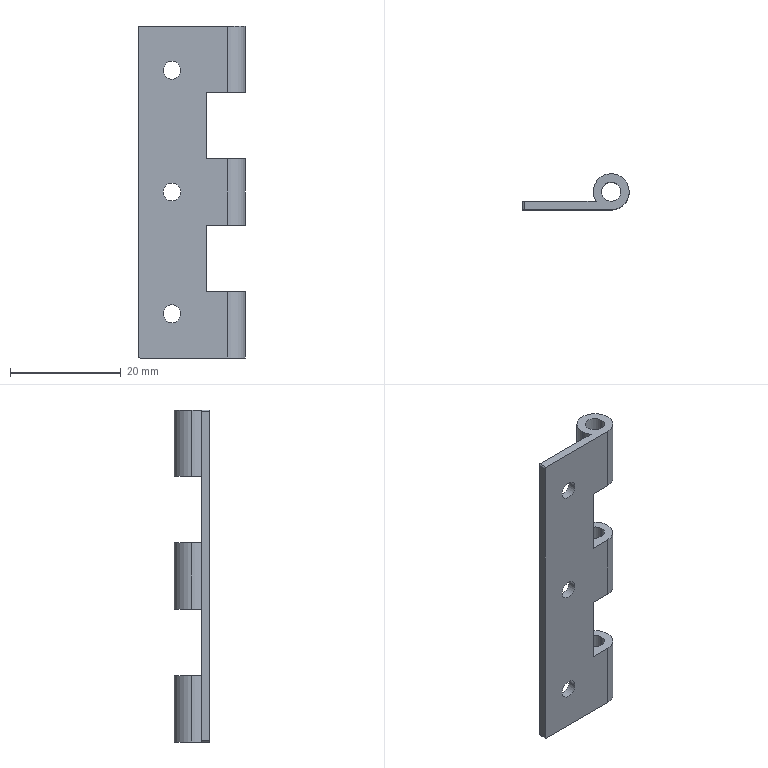Part | STEP file | Second B-1027-14 Pin A Part | 1 solid | 34 faces | box 19.25 x 6.5 x 60 mm | volume 2015 mm3 | cylinder 23 | plane 11 | commonest cylinder face diameters 6.5 x9 3.2 x6 3.5 x6 0.5 x2
STEP:
#1=CARTESIAN_POINT('',(-3.25,0.,-18.));
#2=VERTEX_POINT('',#1);
#3=CARTESIAN_POINT('',(3.25,0.,-18.));
#4=VERTEX_POINT('',#3);
#5=CARTESIAN_POINT('',(0.,0.,-18.));
#6=DIRECTION('',(0.,0.,-1.));
#7=DIRECTION('',(-1.,0.,0.));
#8=AXIS2_PLACEMENT_3D('',#5,#6,#7);
#9=CIRCLE('',#8,3.25);
#10=EDGE_CURVE('',#2,#4,#9,.T.);
#11=ORIENTED_EDGE('',*,*,#10,.T.);
#12=CARTESIAN_POINT('',(3.25,0.,-30.));
#13=VERTEX_POINT('',#12);
#14=CARTESIAN_POINT('',(3.25,0.,30.));
#15=DIRECTION('',(0.,0.,-1.));
#16=VECTOR('',#15,1000.);
#17=LINE('',#14,#16);
#18=EDGE_CURVE('',#4,#13,#17,.T.);
#19=ORIENTED_EDGE('',*,*,#18,.T.);
#20=CARTESIAN_POINT('',(-3.25,0.,-30.));
#21=VERTEX_POINT('',#20);
#22=CARTESIAN_POINT('',(0.,0.,-30.));
#23=DIRECTION('',(0.,0.,1.));
#24=DIRECTION('',(-1.,0.,0.));
#25=AXIS2_PLACEMENT_3D('',#22,#23,#24);
#26=CIRCLE('',#25,3.25);
#27=EDGE_CURVE('',#13,#21,#26,.T.);
#28=ORIENTED_EDGE('',*,*,#27,.T.);
#29=CARTESIAN_POINT('',(-3.25,0.,30.));
#30=DIRECTION('',(0.,0.,-1.));
#31=VECTOR('',#30,1000.);
#32=LINE('',#29,#31);
#33=EDGE_CURVE('',#2,#21,#32,.T.);
#34=ORIENTED_EDGE('',*,*,#33,.F.);
#35=EDGE_LOOP('',(#11,#19,#28,#34));
#36=FACE_OUTER_BOUND('',#35,.T.);
#37=CARTESIAN_POINT('',(0.,0.,30.));
#38=DIRECTION('',(0.,0.,-1.));
#39=DIRECTION('',(-1.,0.,0.));
#40=AXIS2_PLACEMENT_3D('',#37,#38,#39);
#41=CYLINDRICAL_SURFACE('',#40,3.25);
#42=ADVANCED_FACE('',(#36),#41,.T.);
#43=CARTESIAN_POINT('',(-2.739,-1.75,-18.));
#44=VERTEX_POINT('',#43);
#45=CARTESIAN_POINT('',(0.,0.,-18.));
#46=DIRECTION('',(0.,0.,-1.));
#47=DIRECTION('',(-1.,0.,0.));
#48=AXIS2_PLACEMENT_3D('',#45,#46,#47);
#49=CIRCLE('',#48,3.25);
#50=EDGE_CURVE('',#44,#2,#49,.T.);
#51=ORIENTED_EDGE('',*,*,#50,.T.);
#52=ORIENTED_EDGE('',*,*,#33,.T.);
#53=CARTESIAN_POINT('',(-2.739,-1.75,-30.));
#54=VERTEX_POINT('',#53);
#55=CARTESIAN_POINT('',(0.,0.,-30.));
#56=DIRECTION('',(0.,0.,1.));
#57=DIRECTION('',(-1.,0.,0.));
#58=AXIS2_PLACEMENT_3D('',#55,#56,#57);
#59=CIRCLE('',#58,3.25);
#60=EDGE_CURVE('',#21,#54,#59,.T.);
#61=ORIENTED_EDGE('',*,*,#60,.T.);
#62=CARTESIAN_POINT('',(-2.739,-1.75,30.));
#63=DIRECTION('',(0.,0.,1.));
#64=VECTOR('',#63,1000.);
#65=LINE('',#62,#64);
#66=EDGE_CURVE('',#54,#44,#65,.T.);
#67=ORIENTED_EDGE('',*,*,#66,.T.);
#68=EDGE_LOOP('',(#51,#52,#61,#67));
#69=FACE_OUTER_BOUND('',#68,.T.);
#70=CARTESIAN_POINT('',(0.,0.,30.));
#71=DIRECTION('',(0.,0.,-1.));
#72=DIRECTION('',(-1.,0.,0.));
#73=AXIS2_PLACEMENT_3D('',#70,#71,#72);
#74=CYLINDRICAL_SURFACE('',#73,3.25);
#75=ADVANCED_FACE('',(#69),#74,.T.);
#76=CARTESIAN_POINT('',(-3.25,0.,6.));
#77=VERTEX_POINT('',#76);
#78=CARTESIAN_POINT('',(3.25,0.,6.));
#79=VERTEX_POINT('',#78);
#80=CARTESIAN_POINT('',(0.,0.,6.));
#81=DIRECTION('',(0.,0.,-1.));
#82=DIRECTION('',(-1.,0.,0.));
#83=AXIS2_PLACEMENT_3D('',#80,#81,#82);
#84=CIRCLE('',#83,3.25);
#85=EDGE_CURVE('',#77,#79,#84,.T.);
#86=ORIENTED_EDGE('',*,*,#85,.T.);
#87=CARTESIAN_POINT('',(3.25,0.,-6.));
#88=VERTEX_POINT('',#87);
#89=CARTESIAN_POINT('',(3.25,0.,30.));
#90=DIRECTION('',(0.,0.,-1.));
#91=VECTOR('',#90,1000.);
#92=LINE('',#89,#91);
#93=EDGE_CURVE('',#79,#88,#92,.T.);
#94=ORIENTED_EDGE('',*,*,#93,.T.);
#95=CARTESIAN_POINT('',(-3.25,0.,-6.));
#96=VERTEX_POINT('',#95);
#97=CARTESIAN_POINT('',(0.,0.,-6.));
#98=DIRECTION('',(0.,0.,1.));
#99=DIRECTION('',(-1.,0.,0.));
#100=AXIS2_PLACEMENT_3D('',#97,#98,#99);
#101=CIRCLE('',#100,3.25);
#102=EDGE_CURVE('',#88,#96,#101,.T.);
#103=ORIENTED_EDGE('',*,*,#102,.T.);
#104=CARTESIAN_POINT('',(-3.25,0.,30.));
#105=DIRECTION('',(0.,0.,-1.));
#106=VECTOR('',#105,1000.);
#107=LINE('',#104,#106);
#108=EDGE_CURVE('',#77,#96,#107,.T.);
#109=ORIENTED_EDGE('',*,*,#108,.F.);
#110=EDGE_LOOP('',(#86,#94,#103,#109));
#111=FACE_OUTER_BOUND('',#110,.T.);
#112=CARTESIAN_POINT('',(0.,0.,30.));
#113=DIRECTION('',(0.,0.,-1.));
#114=DIRECTION('',(-1.,0.,0.));
#115=AXIS2_PLACEMENT_3D('',#112,#113,#114);
#116=CYLINDRICAL_SURFACE('',#115,3.25);
#117=ADVANCED_FACE('',(#111),#116,.T.);
#118=CARTESIAN_POINT('',(-2.739,-1.75,6.));
#119=VERTEX_POINT('',#118);
#120=CARTESIAN_POINT('',(0.,0.,6.));
#121=DIRECTION('',(0.,0.,-1.));
#122=DIRECTION('',(-1.,0.,0.));
#123=AXIS2_PLACEMENT_3D('',#120,#121,#122);
#124=CIRCLE('',#123,3.25);
#125=EDGE_CURVE('',#119,#77,#124,.T.);
#126=ORIENTED_EDGE('',*,*,#125,.T.);
#127=ORIENTED_EDGE('',*,*,#108,.T.);
#128=CARTESIAN_POINT('',(-2.739,-1.75,-6.));
#129=VERTEX_POINT('',#128);
#130=CARTESIAN_POINT('',(0.,0.,-6.));
#131=DIRECTION('',(0.,0.,1.));
#132=DIRECTION('',(-1.,0.,0.));
#133=AXIS2_PLACEMENT_3D('',#130,#131,#132);
#134=CIRCLE('',#133,3.25);
#135=EDGE_CURVE('',#96,#129,#134,.T.);
#136=ORIENTED_EDGE('',*,*,#135,.T.);
#137=CARTESIAN_POINT('',(-2.739,-1.75,30.));
#138=DIRECTION('',(0.,0.,1.));
#139=VECTOR('',#138,1000.);
#140=LINE('',#137,#139);
#141=EDGE_CURVE('',#129,#119,#140,.T.);
#142=ORIENTED_EDGE('',*,*,#141,.T.);
#143=EDGE_LOOP('',(#126,#127,#136,#142));
#144=FACE_OUTER_BOUND('',#143,.T.);
#145=CARTESIAN_POINT('',(0.,0.,30.));
#146=DIRECTION('',(0.,0.,-1.));
#147=DIRECTION('',(-1.,0.,0.));
#148=AXIS2_PLACEMENT_3D('',#145,#146,#147);
#149=CYLINDRICAL_SURFACE('',#148,3.25);
#150=ADVANCED_FACE('',(#144),#149,.T.);
#151=CARTESIAN_POINT('',(3.25,0.,30.));
#152=VERTEX_POINT('',#151);
#153=CARTESIAN_POINT('',(-3.25,0.,30.));
#154=VERTEX_POINT('',#153);
#155=CARTESIAN_POINT('',(0.,0.,30.));
#156=DIRECTION('',(0.,0.,1.));
#157=DIRECTION('',(-1.,0.,0.));
#158=AXIS2_PLACEMENT_3D('',#155,#156,#157);
#159=CIRCLE('',#158,3.25);
#160=EDGE_CURVE('',#152,#154,#159,.T.);
#161=ORIENTED_EDGE('',*,*,#160,.F.);
#162=CARTESIAN_POINT('',(3.25,0.,18.));
#163=VERTEX_POINT('',#162);
#164=CARTESIAN_POINT('',(3.25,0.,30.));
#165=DIRECTION('',(0.,0.,-1.));
#166=VECTOR('',#165,1000.);
#167=LINE('',#164,#166);
#168=EDGE_CURVE('',#152,#163,#167,.T.);
#169=ORIENTED_EDGE('',*,*,#168,.T.);
#170=CARTESIAN_POINT('',(-3.25,0.,18.));
#171=VERTEX_POINT('',#170);
#172=CARTESIAN_POINT('',(0.,0.,18.));
#173=DIRECTION('',(0.,0.,1.));
#174=DIRECTION('',(-1.,0.,0.));
#175=AXIS2_PLACEMENT_3D('',#172,#173,#174);
#176=CIRCLE('',#175,3.25);
#177=EDGE_CURVE('',#163,#171,#176,.T.);
#178=ORIENTED_EDGE('',*,*,#177,.T.);
#179=CARTESIAN_POINT('',(-3.25,0.,30.));
#180=DIRECTION('',(0.,0.,-1.));
#181=VECTOR('',#180,1000.);
#182=LINE('',#179,#181);
#183=EDGE_CURVE('',#154,#171,#182,.T.);
#184=ORIENTED_EDGE('',*,*,#183,.F.);
#185=EDGE_LOOP('',(#161,#169,#178,#184));
#186=FACE_OUTER_BOUND('',#185,.T.);
#187=CARTESIAN_POINT('',(0.,0.,30.));
#188=DIRECTION('',(0.,0.,-1.));
#189=DIRECTION('',(-1.,0.,0.));
#190=AXIS2_PLACEMENT_3D('',#187,#188,#189);
#191=CYLINDRICAL_SURFACE('',#190,3.25);
#192=ADVANCED_FACE('',(#186),#191,.T.);
#193=CARTESIAN_POINT('',(-2.739,-1.75,30.));
#194=VERTEX_POINT('',#193);
#195=CARTESIAN_POINT('',(0.,0.,30.));
#196=DIRECTION('',(0.,0.,1.));
#197=DIRECTION('',(-1.,0.,0.));
#198=AXIS2_PLACEMENT_3D('',#195,#196,#197);
#199=CIRCLE('',#198,3.25);
#200=EDGE_CURVE('',#154,#194,#199,.T.);
#201=ORIENTED_EDGE('',*,*,#200,.F.);
#202=ORIENTED_EDGE('',*,*,#183,.T.);
#203=CARTESIAN_POINT('',(-2.739,-1.75,18.));
#204=VERTEX_POINT('',#203);
#205=CARTESIAN_POINT('',(0.,0.,18.));
#206=DIRECTION('',(0.,0.,1.));
#207=DIRECTION('',(-1.,0.,0.));
#208=AXIS2_PLACEMENT_3D('',#205,#206,#207);
#209=CIRCLE('',#208,3.25);
#210=EDGE_CURVE('',#171,#204,#209,.T.);
#211=ORIENTED_EDGE('',*,*,#210,.T.);
#212=CARTESIAN_POINT('',(-2.739,-1.75,30.));
#213=DIRECTION('',(0.,0.,1.));
#214=VECTOR('',#213,1000.);
#215=LINE('',#212,#214);
#216=EDGE_CURVE('',#204,#194,#215,.T.);
#217=ORIENTED_EDGE('',*,*,#216,.T.);
#218=EDGE_LOOP('',(#201,#202,#211,#217));
#219=FACE_OUTER_BOUND('',#218,.T.);
#220=CARTESIAN_POINT('',(0.,0.,30.));
#221=DIRECTION('',(0.,0.,-1.));
#222=DIRECTION('',(-1.,0.,0.));
#223=AXIS2_PLACEMENT_3D('',#220,#221,#222);
#224=CYLINDRICAL_SURFACE('',#223,3.25);
#225=ADVANCED_FACE('',(#219),#224,.T.);
#226=CARTESIAN_POINT('',(-11.6,-3.25,-22.));
#227=VERTEX_POINT('',#226);
#228=CARTESIAN_POINT('',(-8.4,-3.25,-22.));
#229=VERTEX_POINT('',#228);
#230=CARTESIAN_POINT('',(-10.,-3.25,-22.));
#231=DIRECTION('',(0.,-1.,0.));
#232=DIRECTION('',(-1.,0.,0.));
#233=AXIS2_PLACEMENT_3D('',#230,#231,#232);
#234=CIRCLE('',#233,1.6);
#235=EDGE_CURVE('',#227,#229,#234,.T.);
#236=ORIENTED_EDGE('',*,*,#235,.T.);
#237=CARTESIAN_POINT('',(-8.4,-1.75,-22.));
#238=VERTEX_POINT('',#237);
#239=CARTESIAN_POINT('',(-8.4,-4.75,-22.));
#240=DIRECTION('',(0.,1.,0.));
#241=VECTOR('',#240,1000.);
#242=LINE('',#239,#241);
#243=EDGE_CURVE('',#229,#238,#242,.T.);
#244=ORIENTED_EDGE('',*,*,#243,.T.);
#245=CARTESIAN_POINT('',(-11.6,-1.75,-22.));
#246=VERTEX_POINT('',#245);
#247=CARTESIAN_POINT('',(-10.,-1.75,-22.));
#248=DIRECTION('',(0.,-1.,0.));
#249=DIRECTION('',(-1.,0.,0.));
#250=AXIS2_PLACEMENT_3D('',#247,#248,#249);
#251=CIRCLE('',#250,1.6);
#252=EDGE_CURVE('',#246,#238,#251,.T.);
#253=ORIENTED_EDGE('',*,*,#252,.F.);
#254=CARTESIAN_POINT('',(-11.6,-4.75,-22.));
#255=DIRECTION('',(0.,1.,0.));
#256=VECTOR('',#255,1000.);
#257=LINE('',#254,#256);
#258=EDGE_CURVE('',#227,#246,#257,.T.);
#259=ORIENTED_EDGE('',*,*,#258,.F.);
#260=EDGE_LOOP('',(#236,#244,#253,#259));
#261=FACE_OUTER_BOUND('',#260,.T.);
#262=CARTESIAN_POINT('',(-10.,-4.75,-22.));
#263=DIRECTION('',(0.,1.,0.));
#264=DIRECTION('',(-1.,0.,0.));
#265=AXIS2_PLACEMENT_3D('',#262,#263,#264);
#266=CYLINDRICAL_SURFACE('',#265,1.6);
#267=ADVANCED_FACE('',(#261),#266,.F.);
#268=CARTESIAN_POINT('',(-11.6,-3.25,0.));
#269=VERTEX_POINT('',#268);
#270=CARTESIAN_POINT('',(-8.4,-3.25,0.));
#271=VERTEX_POINT('',#270);
#272=CARTESIAN_POINT('',(-10.,-3.25,0.));
#273=DIRECTION('',(0.,-1.,0.));
#274=DIRECTION('',(-1.,0.,0.));
#275=AXIS2_PLACEMENT_3D('',#272,#273,#274);
#276=CIRCLE('',#275,1.6);
#277=EDGE_CURVE('',#269,#271,#276,.T.);
#278=ORIENTED_EDGE('',*,*,#277,.T.);
#279=CARTESIAN_POINT('',(-8.4,-1.75,0.));
#280=VERTEX_POINT('',#279);
#281=CARTESIAN_POINT('',(-8.4,-4.75,0.));
#282=DIRECTION('',(0.,1.,0.));
#283=VECTOR('',#282,1000.);
#284=LINE('',#281,#283);
#285=EDGE_CURVE('',#271,#280,#284,.T.);
#286=ORIENTED_EDGE('',*,*,#285,.T.);
#287=CARTESIAN_POINT('',(-11.6,-1.75,0.));
#288=VERTEX_POINT('',#287);
#289=CARTESIAN_POINT('',(-10.,-1.75,0.));
#290=DIRECTION('',(0.,-1.,0.));
#291=DIRECTION('',(-1.,0.,0.));
#292=AXIS2_PLACEMENT_3D('',#289,#290,#291);
#293=CIRCLE('',#292,1.6);
#294=EDGE_CURVE('',#288,#280,#293,.T.);
#295=ORIENTED_EDGE('',*,*,#294,.F.);
#296=CARTESIAN_POINT('',(-11.6,-4.75,0.));
#297=DIRECTION('',(0.,1.,0.));
#298=VECTOR('',#297,1000.);
#299=LINE('',#296,#298);
#300=EDGE_CURVE('',#269,#288,#299,.T.);
#301=ORIENTED_EDGE('',*,*,#300,.F.);
#302=EDGE_LOOP('',(#278,#286,#295,#301));
#303=FACE_OUTER_BOUND('',#302,.T.);
#304=CARTESIAN_POINT('',(-10.,-4.75,0.));
#305=DIRECTION('',(0.,1.,0.));
#306=DIRECTION('',(-1.,0.,0.));
#307=AXIS2_PLACEMENT_3D('',#304,#305,#306);
#308=CYLINDRICAL_SURFACE('',#307,1.6);
#309=ADVANCED_FACE('',(#303),#308,.F.);
#310=CARTESIAN_POINT('',(-11.6,-3.25,22.));
#311=VERTEX_POINT('',#310);
#312=CARTESIAN_POINT('',(-8.4,-3.25,22.));
#313=VERTEX_POINT('',#312);
#314=CARTESIAN_POINT('',(-10.,-3.25,22.));
#315=DIRECTION('',(0.,-1.,0.));
#316=DIRECTION('',(-1.,0.,0.));
#317=AXIS2_PLACEMENT_3D('',#314,#315,#316);
#318=CIRCLE('',#317,1.6);
#319=EDGE_CURVE('',#311,#313,#318,.T.);
#320=ORIENTED_EDGE('',*,*,#319,.T.);
#321=CARTESIAN_POINT('',(-8.4,-1.75,22.));
#322=VERTEX_POINT('',#321);
#323=CARTESIAN_POINT('',(-8.4,-4.75,22.));
#324=DIRECTION('',(0.,1.,0.));
#325=VECTOR('',#324,1000.);
#326=LINE('',#323,#325);
#327=EDGE_CURVE('',#313,#322,#326,.T.);
#328=ORIENTED_EDGE('',*,*,#327,.T.);
#329=CARTESIAN_POINT('',(-11.6,-1.75,22.));
#330=VERTEX_POINT('',#329);
#331=CARTESIAN_POINT('',(-10.,-1.75,22.));
#332=DIRECTION('',(0.,-1.,0.));
#333=DIRECTION('',(-1.,0.,0.));
#334=AXIS2_PLACEMENT_3D('',#331,#332,#333);
#335=CIRCLE('',#334,1.6);
#336=EDGE_CURVE('',#330,#322,#335,.T.);
#337=ORIENTED_EDGE('',*,*,#336,.F.);
#338=CARTESIAN_POINT('',(-11.6,-4.75,22.));
#339=DIRECTION('',(0.,1.,0.));
#340=VECTOR('',#339,1000.);
#341=LINE('',#338,#340);
#342=EDGE_CURVE('',#311,#330,#341,.T.);
#343=ORIENTED_EDGE('',*,*,#342,.F.);
#344=EDGE_LOOP('',(#320,#328,#337,#343));
#345=FACE_OUTER_BOUND('',#344,.T.);
#346=CARTESIAN_POINT('',(-10.,-4.75,22.));
#347=DIRECTION('',(0.,1.,0.));
#348=DIRECTION('',(-1.,0.,0.));
#349=AXIS2_PLACEMENT_3D('',#346,#347,#348);
#350=CYLINDRICAL_SURFACE('',#349,1.6);
#351=ADVANCED_FACE('',(#345),#350,.F.);
#352=CARTESIAN_POINT('',(1.75,0.,30.));
#353=VERTEX_POINT('',#352);
#354=CARTESIAN_POINT('',(-1.75,0.,30.));
#355=VERTEX_POINT('',#354);
#356=CARTESIAN_POINT('',(0.,0.,30.));
#357=DIRECTION('',(0.,0.,-1.));
#358=DIRECTION('',(-1.,0.,0.));
#359=AXIS2_PLACEMENT_3D('',#356,#357,#358);
#360=CIRCLE('',#359,1.75);
#361=EDGE_CURVE('',#353,#355,#360,.T.);
#362=ORIENTED_EDGE('',*,*,#361,.F.);
#363=CARTESIAN_POINT('',(1.75,0.,18.));
#364=VERTEX_POINT('',#363);
#365=CARTESIAN_POINT('',(1.75,0.,30.));
#366=DIRECTION('',(0.,0.,-1.));
#367=VECTOR('',#366,1000.);
#368=LINE('',#365,#367);
#369=EDGE_CURVE('',#353,#364,#368,.T.);
#370=ORIENTED_EDGE('',*,*,#369,.T.);
#371=CARTESIAN_POINT('',(-1.75,0.,18.));
#372=VERTEX_POINT('',#371);
#373=CARTESIAN_POINT('',(0.,0.,18.));
#374=DIRECTION('',(0.,0.,-1.));
#375=DIRECTION('',(-1.,0.,0.));
#376=AXIS2_PLACEMENT_3D('',#373,#374,#375);
#377=CIRCLE('',#376,1.75);
#378=EDGE_CURVE('',#364,#372,#377,.T.);
#379=ORIENTED_EDGE('',*,*,#378,.T.);
#380=CARTESIAN_POINT('',(-1.75,0.,30.));
#381=DIRECTION('',(0.,0.,-1.));
#382=VECTOR('',#381,1000.);
#383=LINE('',#380,#382);
#384=EDGE_CURVE('',#355,#372,#383,.T.);
#385=ORIENTED_EDGE('',*,*,#384,.F.);
#386=EDGE_LOOP('',(#362,#370,#379,#385));
#387=FACE_OUTER_BOUND('',#386,.T.);
#388=CARTESIAN_POINT('',(0.,0.,30.));
#389=DIRECTION('',(0.,0.,-1.));
#390=DIRECTION('',(-1.,0.,0.));
#391=AXIS2_PLACEMENT_3D('',#388,#389,#390);
#392=CYLINDRICAL_SURFACE('',#391,1.75);
#393=ADVANCED_FACE('',(#387),#392,.F.);
#394=CARTESIAN_POINT('',(-1.75,0.,-18.));
#395=VERTEX_POINT('',#394);
#396=CARTESIAN_POINT('',(1.75,0.,-18.));
#397=VERTEX_POINT('',#396);
#398=CARTESIAN_POINT('',(0.,0.,-18.));
#399=DIRECTION('',(0.,0.,1.));
#400=DIRECTION('',(-1.,0.,0.));
#401=AXIS2_PLACEMENT_3D('',#398,#399,#400);
#402=CIRCLE('',#401,1.75);
#403=EDGE_CURVE('',#395,#397,#402,.T.);
#404=ORIENTED_EDGE('',*,*,#403,.T.);
#405=CARTESIAN_POINT('',(1.75,0.,-30.));
#406=VERTEX_POINT('',#405);
#407=CARTESIAN_POINT('',(1.75,0.,30.));
#408=DIRECTION('',(0.,0.,-1.));
#409=VECTOR('',#408,1000.);
#410=LINE('',#407,#409);
#411=EDGE_CURVE('',#397,#406,#410,.T.);
#412=ORIENTED_EDGE('',*,*,#411,.T.);
#413=CARTESIAN_POINT('',(-1.75,0.,-30.));
#414=VERTEX_POINT('',#413);
#415=CARTESIAN_POINT('',(0.,0.,-30.));
#416=DIRECTION('',(0.,0.,-1.));
#417=DIRECTION('',(-1.,0.,0.));
#418=AXIS2_PLACEMENT_3D('',#415,#416,#417);
#419=CIRCLE('',#418,1.75);
#420=EDGE_CURVE('',#406,#414,#419,.T.);
#421=ORIENTED_EDGE('',*,*,#420,.T.);
#422=CARTESIAN_POINT('',(-1.75,0.,30.));
#423=DIRECTION('',(0.,0.,-1.));
#424=VECTOR('',#423,1000.);
#425=LINE('',#422,#424);
#426=EDGE_CURVE('',#395,#414,#425,.T.);
#427=ORIENTED_EDGE('',*,*,#426,.F.);
#428=EDGE_LOOP('',(#404,#412,#421,#427));
#429=FACE_OUTER_BOUND('',#428,.T.);
#430=CARTESIAN_POINT('',(0.,0.,30.));
#431=DIRECTION('',(0.,0.,-1.));
#432=DIRECTION('',(-1.,0.,0.));
#433=AXIS2_PLACEMENT_3D('',#430,#431,#432);
#434=CYLINDRICAL_SURFACE('',#433,1.75);
#435=ADVANCED_FACE('',(#429),#434,.F.);
#436=CARTESIAN_POINT('',(-1.75,0.,6.));
#437=VERTEX_POINT('',#436);
#438=CARTESIAN_POINT('',(1.75,0.,6.));
#439=VERTEX_POINT('',#438);
#440=CARTESIAN_POINT('',(0.,0.,6.));
#441=DIRECTION('',(0.,0.,1.));
#442=DIRECTION('',(-1.,0.,0.));
#443=AXIS2_PLACEMENT_3D('',#440,#441,#442);
#444=CIRCLE('',#443,1.75);
#445=EDGE_CURVE('',#437,#439,#444,.T.);
#446=ORIENTED_EDGE('',*,*,#445,.T.);
#447=CARTESIAN_POINT('',(1.75,0.,-6.));
#448=VERTEX_POINT('',#447);
#449=CARTESIAN_POINT('',(1.75,0.,30.));
#450=DIRECTION('',(0.,0.,-1.));
#451=VECTOR('',#450,1000.);
#452=LINE('',#449,#451);
#453=EDGE_CURVE('',#439,#448,#452,.T.);
#454=ORIENTED_EDGE('',*,*,#453,.T.);
#455=CARTESIAN_POINT('',(-1.75,0.,-6.));
#456=VERTEX_POINT('',#455);
#457=CARTESIAN_POINT('',(0.,0.,-6.));
#458=DIRECTION('',(0.,0.,-1.));
#459=DIRECTION('',(-1.,0.,0.));
#460=AXIS2_PLACEMENT_3D('',#457,#458,#459);
#461=CIRCLE('',#460,1.75);
#462=EDGE_CURVE('',#448,#456,#461,.T.);
#463=ORIENTED_EDGE('',*,*,#462,.T.);
#464=CARTESIAN_POINT('',(-1.75,0.,30.));
#465=DIRECTION('',(0.,0.,-1.));
#466=VECTOR('',#465,1000.);
#467=LINE('',#464,#466);
#468=EDGE_CURVE('',#437,#456,#467,.T.);
#469=ORIENTED_EDGE('',*,*,#468,.F.);
#470=EDGE_LOOP('',(#446,#454,#463,#469));
#471=FACE_OUTER_BOUND('',#470,.T.);
#472=CARTESIAN_POINT('',(0.,0.,30.));
#473=DIRECTION('',(0.,0.,-1.));
#474=DIRECTION('',(-1.,0.,0.));
#475=AXIS2_PLACEMENT_3D('',#472,#473,#474);
#476=CYLINDRICAL_SURFACE('',#475,1.75);
#477=ADVANCED_FACE('',(#471),#476,.F.);
#478=CARTESIAN_POINT('',(-16.,-3.25,29.75));
#479=VERTEX_POINT('',#478);
#480=CARTESIAN_POINT('',(-15.75,-3.25,30.));
#481=VERTEX_POINT('',#480);
#482=CARTESIAN_POINT('',(-15.75,-3.25,29.75));
#483=DIRECTION('',(0.,1.,0.));
#484=DIRECTION('',(0.,0.,1.));
#485=AXIS2_PLACEMENT_3D('',#482,#483,#484);
#486=CIRCLE('',#485,0.25);
#487=EDGE_CURVE('',#479,#481,#486,.T.);
#488=ORIENTED_EDGE('',*,*,#487,.F.);
#489=CARTESIAN_POINT('',(-16.,-3.25,-29.75));
#490=VERTEX_POINT('',#489);
#491=CARTESIAN_POINT('',(-16.,-3.25,30.));
#492=DIRECTION('',(0.,0.,1.));
#493=VECTOR('',#492,1000.);
#494=LINE('',#491,#493);
#495=EDGE_CURVE('',#490,#479,#494,.T.);
#496=ORIENTED_EDGE('',*,*,#495,.F.);
#497=CARTESIAN_POINT('',(-15.75,-3.25,-30.));
#498=VERTEX_POINT('',#497);
#499=CARTESIAN_POINT('',(-15.75,-3.25,-29.75));
#500=DIRECTION('',(0.,1.,0.));
#501=DIRECTION('',(0.,0.,-1.));
#502=AXIS2_PLACEMENT_3D('',#499,#500,#501);
#503=CIRCLE('',#502,0.25);
#504=EDGE_CURVE('',#498,#490,#503,.T.);
#505=ORIENTED_EDGE('',*,*,#504,.F.);
#506=CARTESIAN_POINT('',(0.,-3.25,-30.));
#507=VERTEX_POINT('',#506);
#508=CARTESIAN_POINT('',(0.,-3.25,-30.));
#509=DIRECTION('',(-1.,0.,0.));
#510=VECTOR('',#509,1000.);
#511=LINE('',#508,#510);
#512=EDGE_CURVE('',#507,#498,#511,.T.);
#513=ORIENTED_EDGE('',*,*,#512,.F.);
#514=CARTESIAN_POINT('',(0.,-3.25,-18.));
#515=VERTEX_POINT('',#514);
#516=CARTESIAN_POINT('',(0.,-3.25,30.));
#517=DIRECTION('',(0.,0.,-1.));
#518=VECTOR('',#517,1000.);
#519=LINE('',#516,#518);
#520=EDGE_CURVE('',#515,#507,#519,.T.);
#521=ORIENTED_EDGE('',*,*,#520,.F.);
#522=CARTESIAN_POINT('',(-3.7,-3.25,-18.));
#523=VERTEX_POINT('',#522);
#524=CARTESIAN_POINT('',(0.,-3.25,-18.));
#525=DIRECTION('',(1.,0.,0.));
#526=VECTOR('',#525,1000.);
#527=LINE('',#524,#526);
#528=EDGE_CURVE('',#523,#515,#527,.T.);
#529=ORIENTED_EDGE('',*,*,#528,.F.);
#530=CARTESIAN_POINT('',(-3.7,-3.25,-6.));
#531=VERTEX_POINT('',#530);
#532=CARTESIAN_POINT('',(-3.7,-3.25,30.));
#533=DIRECTION('',(0.,0.,-1.));
#534=VECTOR('',#533,1000.);
#535=LINE('',#532,#534);
#536=EDGE_CURVE('',#531,#523,#535,.T.);
#537=ORIENTED_EDGE('',*,*,#536,.F.);
#538=CARTESIAN_POINT('',(0.,-3.25,-6.));
#539=VERTEX_POINT('',#538);
#540=CARTESIAN_POINT('',(0.,-3.25,-6.));
#541=DIRECTION('',(-1.,0.,0.));
#542=VECTOR('',#541,1000.);
#543=LINE('',#540,#542);
#544=EDGE_CURVE('',#539,#531,#543,.T.);
#545=ORIENTED_EDGE('',*,*,#544,.F.);
#546=CARTESIAN_POINT('',(0.,-3.25,6.));
#547=VERTEX_POINT('',#546);
#548=CARTESIAN_POINT('',(0.,-3.25,30.));
#549=DIRECTION('',(0.,0.,-1.));
#550=VECTOR('',#549,1000.);
#551=LINE('',#548,#550);
#552=EDGE_CURVE('',#547,#539,#551,.T.);
#553=ORIENTED_EDGE('',*,*,#552,.F.);
#554=CARTESIAN_POINT('',(-3.7,-3.25,6.));
#555=VERTEX_POINT('',#554);
#556=CARTESIAN_POINT('',(0.,-3.25,6.));
#557=DIRECTION('',(1.,0.,0.));
#558=VECTOR('',#557,1000.);
#559=LINE('',#556,#558);
#560=EDGE_CURVE('',#555,#547,#559,.T.);
#561=ORIENTED_EDGE('',*,*,#560,.F.);
#562=CARTESIAN_POINT('',(-3.7,-3.25,18.));
#563=VERTEX_POINT('',#562);
#564=CARTESIAN_POINT('',(-3.7,-3.25,30.));
#565=DIRECTION('',(0.,0.,-1.));
#566=VECTOR('',#565,1000.);
#567=LINE('',#564,#566);
#568=EDGE_CURVE('',#563,#555,#567,.T.);
#569=ORIENTED_EDGE('',*,*,#568,.F.);
#570=CARTESIAN_POINT('',(0.,-3.25,18.));
#571=VERTEX_POINT('',#570);
#572=CARTESIAN_POINT('',(0.,-3.25,18.));
#573=DIRECTION('',(-1.,0.,0.));
#574=VECTOR('',#573,1000.);
#575=LINE('',#572,#574);
#576=EDGE_CURVE('',#571,#563,#575,.T.);
#577=ORIENTED_EDGE('',*,*,#576,.F.);
#578=CARTESIAN_POINT('',(0.,-3.25,30.));
#579=VERTEX_POINT('',#578);
#580=CARTESIAN_POINT('',(0.,-3.25,30.));
#581=DIRECTION('',(0.,0.,-1.));
#582=VECTOR('',#581,1000.);
#583=LINE('',#580,#582);
#584=EDGE_CURVE('',#579,#571,#583,.T.);
#585=ORIENTED_EDGE('',*,*,#584,.F.);
#586=CARTESIAN_POINT('',(0.,-3.25,30.));
#587=DIRECTION('',(1.,0.,0.));
#588=VECTOR('',#587,1000.);
#589=LINE('',#586,#588);
#590=EDGE_CURVE('',#481,#579,#589,.T.);
#591=ORIENTED_EDGE('',*,*,#590,.F.);
#592=EDGE_LOOP('',(#488,#496,#505,#513,#521,#529,#537,#545,#553,#561,#569,#577,#585,#591));
#593=FACE_OUTER_BOUND('',#592,.T.);
#594=ORIENTED_EDGE('',*,*,#235,.F.);
#595=CARTESIAN_POINT('',(-10.,-3.25,-22.));
#596=DIRECTION('',(0.,-1.,0.));
#597=DIRECTION('',(-1.,0.,0.));
#598=AXIS2_PLACEMENT_3D('',#595,#596,#597);
#599=CIRCLE('',#598,1.6);
#600=EDGE_CURVE('',#229,#227,#599,.T.);
#601=ORIENTED_EDGE('',*,*,#600,.F.);
#602=EDGE_LOOP('',(#594,#601));
#603=FACE_BOUND('',#602,.T.);
#604=ORIENTED_EDGE('',*,*,#277,.F.);
#605=CARTESIAN_POINT('',(-10.,-3.25,0.));
#606=DIRECTION('',(0.,-1.,0.));
#607=DIRECTION('',(-1.,0.,0.));
#608=AXIS2_PLACEMENT_3D('',#605,#606,#607);
#609=CIRCLE('',#608,1.6);
#610=EDGE_CURVE('',#271,#269,#609,.T.);
#611=ORIENTED_EDGE('',*,*,#610,.F.);
#612=EDGE_LOOP('',(#604,#611));
#613=FACE_BOUND('',#612,.T.);
#614=ORIENTED_EDGE('',*,*,#319,.F.);
#615=CARTESIAN_POINT('',(-10.,-3.25,22.));
#616=DIRECTION('',(0.,-1.,0.));
#617=DIRECTION('',(-1.,0.,0.));
#618=AXIS2_PLACEMENT_3D('',#615,#616,#617);
#619=CIRCLE('',#618,1.6);
#620=EDGE_CURVE('',#313,#311,#619,.T.);
#621=ORIENTED_EDGE('',*,*,#620,.F.);
#622=EDGE_LOOP('',(#614,#621));
#623=FACE_BOUND('',#622,.T.);
#624=CARTESIAN_POINT('',(0.,-3.25,30.));
#625=DIRECTION('',(0.,1.,0.));
#626=DIRECTION('',(-1.,0.,0.));
#627=AXIS2_PLACEMENT_3D('',#624,#625,#626);
#628=PLANE('',#627);
#629=ADVANCED_FACE('',(#593,#603,#613,#623),#628,.F.);
#630=CARTESIAN_POINT('',(0.,0.,30.));
#631=DIRECTION('',(0.,0.,-1.));
#632=DIRECTION('',(-1.,0.,0.));
#633=AXIS2_PLACEMENT_3D('',#630,#631,#632);
#634=CIRCLE('',#633,1.75);
#635=EDGE_CURVE('',#355,#353,#634,.T.);
#636=ORIENTED_EDGE('',*,*,#635,.T.);
#637=ORIENTED_EDGE('',*,*,#361,.T.);
#638=EDGE_LOOP('',(#636,#637));
#639=FACE_BOUND('',#638,.T.);
#640=ORIENTED_EDGE('',*,*,#590,.T.);
#641=CARTESIAN_POINT('',(0.,0.,30.));
#642=DIRECTION('',(0.,0.,1.));
#643=DIRECTION('',(-1.,0.,0.));
#644=AXIS2_PLACEMENT_3D('',#641,#642,#643);
#645=CIRCLE('',#644,3.25);
#646=EDGE_CURVE('',#579,#152,#645,.T.);
#647=ORIENTED_EDGE('',*,*,#646,.T.);
#648=ORIENTED_EDGE('',*,*,#160,.T.);
#649=ORIENTED_EDGE('',*,*,#200,.T.);
#650=CARTESIAN_POINT('',(-15.75,-1.75,30.));
#651=VERTEX_POINT('',#650);
#652=CARTESIAN_POINT('',(0.,-1.75,30.));
#653=DIRECTION('',(-1.,0.,0.));
#654=VECTOR('',#653,1000.);
#655=LINE('',#652,#654);
#656=EDGE_CURVE('',#194,#651,#655,.T.);
#657=ORIENTED_EDGE('',*,*,#656,.T.);
#658=CARTESIAN_POINT('',(-15.75,0.,30.));
#659=DIRECTION('',(0.,-1.,0.));
#660=VECTOR('',#659,1000.);
#661=LINE('',#658,#660);
#662=EDGE_CURVE('',#651,#481,#661,.T.);
#663=ORIENTED_EDGE('',*,*,#662,.T.);
#664=EDGE_LOOP('',(#640,#647,#648,#649,#657,#663));
#665=FACE_OUTER_BOUND('',#664,.T.);
#666=CARTESIAN_POINT('',(0.,0.,30.));
#667=DIRECTION('',(0.,0.,1.));
#668=DIRECTION('',(1.,0.,0.));
#669=AXIS2_PLACEMENT_3D('',#666,#667,#668);
#670=PLANE('',#669);
#671=ADVANCED_FACE('',(#639,#665),#670,.T.);
#672=CARTESIAN_POINT('',(-16.,-1.75,29.75));
#673=VERTEX_POINT('',#672);
#674=CARTESIAN_POINT('',(-16.,-3.25,29.75));
#675=DIRECTION('',(0.,-1.,0.));
#676=VECTOR('',#675,1000.);
#677=LINE('',#674,#676);
#678=EDGE_CURVE('',#673,#479,#677,.T.);
#679=ORIENTED_EDGE('',*,*,#678,.F.);
#680=CARTESIAN_POINT('',(-16.,-1.75,-29.75));
#681=VERTEX_POINT('',#680);
#682=CARTESIAN_POINT('',(-16.,-1.75,30.));
#683=DIRECTION('',(0.,0.,1.));
#684=VECTOR('',#683,1000.);
#685=LINE('',#682,#684);
#686=EDGE_CURVE('',#681,#673,#685,.T.);
#687=ORIENTED_EDGE('',*,*,#686,.F.);
#688=CARTESIAN_POINT('',(-16.,-3.25,-29.75));
#689=DIRECTION('',(0.,1.,0.));
#690=VECTOR('',#689,1000.);
#691=LINE('',#688,#690);
#692=EDGE_CURVE('',#490,#681,#691,.T.);
#693=ORIENTED_EDGE('',*,*,#692,.F.);
#694=ORIENTED_EDGE('',*,*,#495,.T.);
#695=EDGE_LOOP('',(#679,#687,#693,#694));
#696=FACE_OUTER_BOUND('',#695,.T.);
#697=CARTESIAN_POINT('',(-16.,-3.25,30.));
#698=DIRECTION('',(1.,0.,0.));
#699=DIRECTION('',(0.,0.,-1.));
#700=AXIS2_PLACEMENT_3D('',#697,#698,#699);
#701=PLANE('',#700);
#702=ADVANCED_FACE('',(#696),#701,.F.);
#703=CARTESIAN_POINT('',(0.,0.,-30.));
#704=DIRECTION('',(0.,0.,-1.));
#705=DIRECTION('',(-1.,0.,0.));
#706=AXIS2_PLACEMENT_3D('',#703,#704,#705);
#707=CIRCLE('',#706,1.75);
#708=EDGE_CURVE('',#414,#406,#707,.T.);
#709=ORIENTED_EDGE('',*,*,#708,.F.);
#710=ORIENTED_EDGE('',*,*,#420,.F.);
#711=EDGE_LOOP('',(#709,#710));
#712=FACE_BOUND('',#711,.T.);
#713=CARTESIAN_POINT('',(-15.75,-1.75,-30.));
#714=VERTEX_POINT('',#713);
#715=CARTESIAN_POINT('',(-15.75,0.,-30.));
#716=DIRECTION('',(0.,-1.,0.));
#717=VECTOR('',#716,1000.);
#718=LINE('',#715,#717);
#719=EDGE_CURVE('',#714,#498,#718,.T.);
#720=ORIENTED_EDGE('',*,*,#719,.F.);
#721=CARTESIAN_POINT('',(0.,-1.75,-30.));
#722=DIRECTION('',(-1.,0.,0.));
#723=VECTOR('',#722,1000.);
#724=LINE('',#721,#723);
#725=EDGE_CURVE('',#54,#714,#724,.T.);
#726=ORIENTED_EDGE('',*,*,#725,.F.);
#727=ORIENTED_EDGE('',*,*,#60,.F.);
#728=ORIENTED_EDGE('',*,*,#27,.F.);
#729=CARTESIAN_POINT('',(0.,0.,-30.));
#730=DIRECTION('',(0.,0.,1.));
#731=DIRECTION('',(-1.,0.,0.));
#732=AXIS2_PLACEMENT_3D('',#729,#730,#731);
#733=CIRCLE('',#732,3.25);
#734=EDGE_CURVE('',#507,#13,#733,.T.);
#735=ORIENTED_EDGE('',*,*,#734,.F.);
#736=ORIENTED_EDGE('',*,*,#512,.T.);
#737=EDGE_LOOP('',(#720,#726,#727,#728,#735,#736));
#738=FACE_OUTER_BOUND('',#737,.T.);
#739=CARTESIAN_POINT('',(0.,0.,-30.));
#740=DIRECTION('',(0.,0.,1.));
#741=DIRECTION('',(1.,0.,0.));
#742=AXIS2_PLACEMENT_3D('',#739,#740,#741);
#743=PLANE('',#742);
#744=ADVANCED_FACE('',(#712,#738),#743,.F.);
#745=ORIENTED_EDGE('',*,*,#18,.F.);
#746=CARTESIAN_POINT('',(0.,0.,-18.));
#747=DIRECTION('',(0.,0.,-1.));
#748=DIRECTION('',(-1.,0.,0.));
#749=AXIS2_PLACEMENT_3D('',#746,#747,#748);
#750=CIRCLE('',#749,3.25);
#751=EDGE_CURVE('',#4,#515,#750,.T.);
#752=ORIENTED_EDGE('',*,*,#751,.T.);
#753=ORIENTED_EDGE('',*,*,#520,.T.);
#754=ORIENTED_EDGE('',*,*,#734,.T.);
#755=EDGE_LOOP('',(#745,#752,#753,#754));
#756=FACE_OUTER_BOUND('',#755,.T.);
#757=CARTESIAN_POINT('',(0.,0.,30.));
#758=DIRECTION('',(0.,0.,-1.));
#759=DIRECTION('',(-1.,0.,0.));
#760=AXIS2_PLACEMENT_3D('',#757,#758,#759);
#761=CYLINDRICAL_SURFACE('',#760,3.25);
#762=ADVANCED_FACE('',(#756),#761,.T.);
#763=ORIENTED_EDGE('',*,*,#528,.T.);
#764=ORIENTED_EDGE('',*,*,#751,.F.);
#765=ORIENTED_EDGE('',*,*,#10,.F.);
#766=ORIENTED_EDGE('',*,*,#50,.F.);
#767=CARTESIAN_POINT('',(-3.7,-1.75,-18.));
#768=VERTEX_POINT('',#767);
#769=CARTESIAN_POINT('',(3.25,-1.75,-18.));
#770=DIRECTION('',(1.,0.,0.));
#771=VECTOR('',#770,1000.);
#772=LINE('',#769,#771);
#773=EDGE_CURVE('',#768,#44,#772,.T.);
#774=ORIENTED_EDGE('',*,*,#773,.F.);
#775=CARTESIAN_POINT('',(-3.7,-31.75,-18.));
#776=DIRECTION('',(0.,1.,0.));
#777=VECTOR('',#776,1000.);
#778=LINE('',#775,#777);
#779=EDGE_CURVE('',#523,#768,#778,.T.);
#780=ORIENTED_EDGE('',*,*,#779,.F.);
#781=EDGE_LOOP('',(#763,#764,#765,#766,#774,#780));
#782=FACE_OUTER_BOUND('',#781,.T.);
#783=ORIENTED_EDGE('',*,*,#403,.F.);
#784=CARTESIAN_POINT('',(0.,0.,-18.));
#785=DIRECTION('',(0.,0.,1.));
#786=DIRECTION('',(-1.,0.,0.));
#787=AXIS2_PLACEMENT_3D('',#784,#785,#786);
#788=CIRCLE('',#787,1.75);
#789=EDGE_CURVE('',#397,#395,#788,.T.);
#790=ORIENTED_EDGE('',*,*,#789,.F.);
#791=EDGE_LOOP('',(#783,#790));
#792=FACE_BOUND('',#791,.T.);
#793=CARTESIAN_POINT('',(3.25,-31.75,-18.));
#794=DIRECTION('',(0.,0.,-1.));
#795=DIRECTION('',(-1.,0.,0.));
#796=AXIS2_PLACEMENT_3D('',#793,#794,#795);
#797=PLANE('',#796);
#798=ADVANCED_FACE('',(#782,#792),#797,.F.);
#799=ORIENTED_EDGE('',*,*,#536,.T.);
#800=ORIENTED_EDGE('',*,*,#779,.T.);
#801=CARTESIAN_POINT('',(-3.7,-1.75,-6.));
#802=VERTEX_POINT('',#801);
#803=CARTESIAN_POINT('',(-3.7,-1.75,-18.));
#804=DIRECTION('',(0.,0.,-1.));
#805=VECTOR('',#804,1000.);
#806=LINE('',#803,#805);
#807=EDGE_CURVE('',#802,#768,#806,.T.);
#808=ORIENTED_EDGE('',*,*,#807,.F.);
#809=CARTESIAN_POINT('',(-3.7,-31.75,-6.));
#810=DIRECTION('',(0.,1.,0.));
#811=VECTOR('',#810,1000.);
#812=LINE('',#809,#811);
#813=EDGE_CURVE('',#531,#802,#812,.T.);
#814=ORIENTED_EDGE('',*,*,#813,.F.);
#815=EDGE_LOOP('',(#799,#800,#808,#814));
#816=FACE_OUTER_BOUND('',#815,.T.);
#817=CARTESIAN_POINT('',(-3.7,-31.75,-18.));
#818=DIRECTION('',(-1.,0.,0.));
#819=DIRECTION('',(0.,0.,1.));
#820=AXIS2_PLACEMENT_3D('',#817,#818,#819);
#821=PLANE('',#820);
#822=ADVANCED_FACE('',(#816),#821,.F.);
#823=ORIENTED_EDGE('',*,*,#544,.T.);
#824=ORIENTED_EDGE('',*,*,#813,.T.);
#825=CARTESIAN_POINT('',(3.25,-1.75,-6.));
#826=DIRECTION('',(-1.,0.,0.));
#827=VECTOR('',#826,1000.);
#828=LINE('',#825,#827);
#829=EDGE_CURVE('',#129,#802,#828,.T.);
#830=ORIENTED_EDGE('',*,*,#829,.F.);
#831=ORIENTED_EDGE('',*,*,#135,.F.);
#832=ORIENTED_EDGE('',*,*,#102,.F.);
#833=CARTESIAN_POINT('',(0.,0.,-6.));
#834=DIRECTION('',(0.,0.,1.));
#835=DIRECTION('',(-1.,0.,0.));
#836=AXIS2_PLACEMENT_3D('',#833,#834,#835);
#837=CIRCLE('',#836,3.25);
#838=EDGE_CURVE('',#539,#88,#837,.T.);
#839=ORIENTED_EDGE('',*,*,#838,.F.);
#840=EDGE_LOOP('',(#823,#824,#830,#831,#832,#839));
#841=FACE_OUTER_BOUND('',#840,.T.);
#842=CARTESIAN_POINT('',(0.,0.,-6.));
#843=DIRECTION('',(0.,0.,-1.));
#844=DIRECTION('',(-1.,0.,0.));
#845=AXIS2_PLACEMENT_3D('',#842,#843,#844);
#846=CIRCLE('',#845,1.75);
#847=EDGE_CURVE('',#456,#448,#846,.T.);
#848=ORIENTED_EDGE('',*,*,#847,.F.);
#849=ORIENTED_EDGE('',*,*,#462,.F.);
#850=EDGE_LOOP('',(#848,#849));
#851=FACE_BOUND('',#850,.T.);
#852=CARTESIAN_POINT('',(3.25,-31.75,-6.));
#853=DIRECTION('',(0.,0.,1.));
#854=DIRECTION('',(1.,0.,0.));
#855=AXIS2_PLACEMENT_3D('',#852,#853,#854);
#856=PLANE('',#855);
#857=ADVANCED_FACE('',(#841,#851),#856,.F.);
#858=ORIENTED_EDGE('',*,*,#93,.F.);
#859=CARTESIAN_POINT('',(0.,0.,6.));
#860=DIRECTION('',(0.,0.,-1.));
#861=DIRECTION('',(-1.,0.,0.));
#862=AXIS2_PLACEMENT_3D('',#859,#860,#861);
#863=CIRCLE('',#862,3.25);
#864=EDGE_CURVE('',#79,#547,#863,.T.);
#865=ORIENTED_EDGE('',*,*,#864,.T.);
#866=ORIENTED_EDGE('',*,*,#552,.T.);
#867=ORIENTED_EDGE('',*,*,#838,.T.);
#868=EDGE_LOOP('',(#858,#865,#866,#867));
#869=FACE_OUTER_BOUND('',#868,.T.);
#870=CARTESIAN_POINT('',(0.,0.,30.));
#871=DIRECTION('',(0.,0.,-1.));
#872=DIRECTION('',(-1.,0.,0.));
#873=AXIS2_PLACEMENT_3D('',#870,#871,#872);
#874=CYLINDRICAL_SURFACE('',#873,3.25);
#875=ADVANCED_FACE('',(#869),#874,.T.);
#876=ORIENTED_EDGE('',*,*,#560,.T.);
#877=ORIENTED_EDGE('',*,*,#864,.F.);
#878=ORIENTED_EDGE('',*,*,#85,.F.);
#879=ORIENTED_EDGE('',*,*,#125,.F.);
#880=CARTESIAN_POINT('',(-3.7,-1.75,6.));
#881=VERTEX_POINT('',#880);
#882=CARTESIAN_POINT('',(3.25,-1.75,6.));
#883=DIRECTION('',(1.,0.,0.));
#884=VECTOR('',#883,1000.);
#885=LINE('',#882,#884);
#886=EDGE_CURVE('',#881,#119,#885,.T.);
#887=ORIENTED_EDGE('',*,*,#886,.F.);
#888=CARTESIAN_POINT('',(-3.7,-31.75,6.));
#889=DIRECTION('',(0.,1.,0.));
#890=VECTOR('',#889,1000.);
#891=LINE('',#888,#890);
#892=EDGE_CURVE('',#555,#881,#891,.T.);
#893=ORIENTED_EDGE('',*,*,#892,.F.);
#894=EDGE_LOOP('',(#876,#877,#878,#879,#887,#893));
#895=FACE_OUTER_BOUND('',#894,.T.);
#896=ORIENTED_EDGE('',*,*,#445,.F.);
#897=CARTESIAN_POINT('',(0.,0.,6.));
#898=DIRECTION('',(0.,0.,1.));
#899=DIRECTION('',(-1.,0.,0.));
#900=AXIS2_PLACEMENT_3D('',#897,#898,#899);
#901=CIRCLE('',#900,1.75);
#902=EDGE_CURVE('',#439,#437,#901,.T.);
#903=ORIENTED_EDGE('',*,*,#902,.F.);
#904=EDGE_LOOP('',(#896,#903));
#905=FACE_BOUND('',#904,.T.);
#906=CARTESIAN_POINT('',(3.25,-31.75,6.));
#907=DIRECTION('',(0.,0.,-1.));
#908=DIRECTION('',(-1.,0.,0.));
#909=AXIS2_PLACEMENT_3D('',#906,#907,#908);
#910=PLANE('',#909);
#911=ADVANCED_FACE('',(#895,#905),#910,.F.);
#912=ORIENTED_EDGE('',*,*,#568,.T.);
#913=ORIENTED_EDGE('',*,*,#892,.T.);
#914=CARTESIAN_POINT('',(-3.7,-1.75,18.));
#915=VERTEX_POINT('',#914);
#916=CARTESIAN_POINT('',(-3.7,-1.75,6.));
#917=DIRECTION('',(0.,0.,-1.));
#918=VECTOR('',#917,1000.);
#919=LINE('',#916,#918);
#920=EDGE_CURVE('',#915,#881,#919,.T.);
#921=ORIENTED_EDGE('',*,*,#920,.F.);
#922=CARTESIAN_POINT('',(-3.7,-31.75,18.));
#923=DIRECTION('',(0.,1.,0.));
#924=VECTOR('',#923,1000.);
#925=LINE('',#922,#924);
#926=EDGE_CURVE('',#563,#915,#925,.T.);
#927=ORIENTED_EDGE('',*,*,#926,.F.);
#928=EDGE_LOOP('',(#912,#913,#921,#927));
#929=FACE_OUTER_BOUND('',#928,.T.);
#930=CARTESIAN_POINT('',(-3.7,-31.75,6.));
#931=DIRECTION('',(-1.,0.,0.));
#932=DIRECTION('',(0.,0.,1.));
#933=AXIS2_PLACEMENT_3D('',#930,#931,#932);
#934=PLANE('',#933);
#935=ADVANCED_FACE('',(#929),#934,.F.);
#936=ORIENTED_EDGE('',*,*,#576,.T.);
#937=ORIENTED_EDGE('',*,*,#926,.T.);
#938=CARTESIAN_POINT('',(3.25,-1.75,18.));
#939=DIRECTION('',(-1.,0.,0.));
#940=VECTOR('',#939,1000.);
#941=LINE('',#938,#940);
#942=EDGE_CURVE('',#204,#915,#941,.T.);
#943=ORIENTED_EDGE('',*,*,#942,.F.);
#944=ORIENTED_EDGE('',*,*,#210,.F.);
#945=ORIENTED_EDGE('',*,*,#177,.F.);
#946=CARTESIAN_POINT('',(0.,0.,18.));
#947=DIRECTION('',(0.,0.,1.));
#948=DIRECTION('',(-1.,0.,0.));
#949=AXIS2_PLACEMENT_3D('',#946,#947,#948);
#950=CIRCLE('',#949,3.25);
#951=EDGE_CURVE('',#571,#163,#950,.T.);
#952=ORIENTED_EDGE('',*,*,#951,.F.);
#953=EDGE_LOOP('',(#936,#937,#943,#944,#945,#952));
#954=FACE_OUTER_BOUND('',#953,.T.);
#955=CARTESIAN_POINT('',(0.,0.,18.));
#956=DIRECTION('',(0.,0.,-1.));
#957=DIRECTION('',(-1.,0.,0.));
#958=AXIS2_PLACEMENT_3D('',#955,#956,#957);
#959=CIRCLE('',#958,1.75);
#960=EDGE_CURVE('',#372,#364,#959,.T.);
#961=ORIENTED_EDGE('',*,*,#960,.F.);
#962=ORIENTED_EDGE('',*,*,#378,.F.);
#963=EDGE_LOOP('',(#961,#962));
#964=FACE_BOUND('',#963,.T.);
#965=CARTESIAN_POINT('',(3.25,-31.75,18.));
#966=DIRECTION('',(0.,0.,1.));
#967=DIRECTION('',(1.,0.,0.));
#968=AXIS2_PLACEMENT_3D('',#965,#966,#967);
#969=PLANE('',#968);
#970=ADVANCED_FACE('',(#954,#964),#969,.F.);
#971=ORIENTED_EDGE('',*,*,#168,.F.);
#972=ORIENTED_EDGE('',*,*,#646,.F.);
#973=ORIENTED_EDGE('',*,*,#584,.T.);
#974=ORIENTED_EDGE('',*,*,#951,.T.);
#975=EDGE_LOOP('',(#971,#972,#973,#974));
#976=FACE_OUTER_BOUND('',#975,.T.);
#977=CARTESIAN_POINT('',(0.,0.,30.));
#978=DIRECTION('',(0.,0.,-1.));
#979=DIRECTION('',(-1.,0.,0.));
#980=AXIS2_PLACEMENT_3D('',#977,#978,#979);
#981=CYLINDRICAL_SURFACE('',#980,3.25);
#982=ADVANCED_FACE('',(#976),#981,.T.);
#983=ORIENTED_EDGE('',*,*,#243,.F.);
#984=ORIENTED_EDGE('',*,*,#600,.T.);
#985=ORIENTED_EDGE('',*,*,#258,.T.);
#986=CARTESIAN_POINT('',(-10.,-1.75,-22.));
#987=DIRECTION('',(0.,-1.,0.));
#988=DIRECTION('',(-1.,0.,0.));
#989=AXIS2_PLACEMENT_3D('',#986,#987,#988);
#990=CIRCLE('',#989,1.6);
#991=EDGE_CURVE('',#238,#246,#990,.T.);
#992=ORIENTED_EDGE('',*,*,#991,.F.);
#993=EDGE_LOOP('',(#983,#984,#985,#992));
#994=FACE_OUTER_BOUND('',#993,.T.);
#995=CARTESIAN_POINT('',(-10.,-4.75,-22.));
#996=DIRECTION('',(0.,1.,0.));
#997=DIRECTION('',(-1.,0.,0.));
#998=AXIS2_PLACEMENT_3D('',#995,#996,#997);
#999=CYLINDRICAL_SURFACE('',#998,1.6);
#1000=ADVANCED_FACE('',(#994),#999,.F.);
#1001=ORIENTED_EDGE('',*,*,#285,.F.);
#1002=ORIENTED_EDGE('',*,*,#610,.T.);
#1003=ORIENTED_EDGE('',*,*,#300,.T.);
#1004=CARTESIAN_POINT('',(-10.,-1.75,0.));
#1005=DIRECTION('',(0.,-1.,0.));
#1006=DIRECTION('',(-1.,0.,0.));
#1007=AXIS2_PLACEMENT_3D('',#1004,#1005,#1006);
#1008=CIRCLE('',#1007,1.6);
#1009=EDGE_CURVE('',#280,#288,#1008,.T.);
#1010=ORIENTED_EDGE('',*,*,#1009,.F.);
#1011=EDGE_LOOP('',(#1001,#1002,#1003,#1010));
#1012=FACE_OUTER_BOUND('',#1011,.T.);
#1013=CARTESIAN_POINT('',(-10.,-4.75,0.));
#1014=DIRECTION('',(0.,1.,0.));
#1015=DIRECTION('',(-1.,0.,0.));
#1016=AXIS2_PLACEMENT_3D('',#1013,#1014,#1015);
#1017=CYLINDRICAL_SURFACE('',#1016,1.6);
#1018=ADVANCED_FACE('',(#1012),#1017,.F.);
#1019=ORIENTED_EDGE('',*,*,#327,.F.);
#1020=ORIENTED_EDGE('',*,*,#620,.T.);
#1021=ORIENTED_EDGE('',*,*,#342,.T.);
#1022=CARTESIAN_POINT('',(-10.,-1.75,22.));
#1023=DIRECTION('',(0.,-1.,0.));
#1024=DIRECTION('',(-1.,0.,0.));
#1025=AXIS2_PLACEMENT_3D('',#1022,#1023,#1024);
#1026=CIRCLE('',#1025,1.6);
#1027=EDGE_CURVE('',#322,#330,#1026,.T.);
#1028=ORIENTED_EDGE('',*,*,#1027,.F.);
#1029=EDGE_LOOP('',(#1019,#1020,#1021,#1028));
#1030=FACE_OUTER_BOUND('',#1029,.T.);
#1031=CARTESIAN_POINT('',(-10.,-4.75,22.));
#1032=DIRECTION('',(0.,1.,0.));
#1033=DIRECTION('',(-1.,0.,0.));
#1034=AXIS2_PLACEMENT_3D('',#1031,#1032,#1033);
#1035=CYLINDRICAL_SURFACE('',#1034,1.6);
#1036=ADVANCED_FACE('',(#1030),#1035,.F.);
#1037=ORIENTED_EDGE('',*,*,#369,.F.);
#1038=ORIENTED_EDGE('',*,*,#635,.F.);
#1039=ORIENTED_EDGE('',*,*,#384,.T.);
#1040=ORIENTED_EDGE('',*,*,#960,.T.);
#1041=EDGE_LOOP('',(#1037,#1038,#1039,#1040));
#1042=FACE_OUTER_BOUND('',#1041,.T.);
#1043=CARTESIAN_POINT('',(0.,0.,30.));
#1044=DIRECTION('',(0.,0.,-1.));
#1045=DIRECTION('',(-1.,0.,0.));
#1046=AXIS2_PLACEMENT_3D('',#1043,#1044,#1045);
#1047=CYLINDRICAL_SURFACE('',#1046,1.75);
#1048=ADVANCED_FACE('',(#1042),#1047,.F.);
#1049=ORIENTED_EDGE('',*,*,#487,.T.);
#1050=ORIENTED_EDGE('',*,*,#662,.F.);
#1051=CARTESIAN_POINT('',(-15.75,-1.75,29.75));
#1052=DIRECTION('',(0.,-1.,0.));
#1053=DIRECTION('',(0.,0.,1.));
#1054=AXIS2_PLACEMENT_3D('',#1051,#1052,#1053);
#1055=CIRCLE('',#1054,0.25);
#1056=EDGE_CURVE('',#651,#673,#1055,.T.);
#1057=ORIENTED_EDGE('',*,*,#1056,.T.);
#1058=ORIENTED_EDGE('',*,*,#678,.T.);
#1059=EDGE_LOOP('',(#1049,#1050,#1057,#1058));
#1060=FACE_OUTER_BOUND('',#1059,.T.);
#1061=CARTESIAN_POINT('',(-15.75,0.,29.75));
#1062=DIRECTION('',(0.,1.,0.));
#1063=DIRECTION('',(0.,0.,1.));
#1064=AXIS2_PLACEMENT_3D('',#1061,#1062,#1063);
#1065=CYLINDRICAL_SURFACE('',#1064,0.25);
#1066=ADVANCED_FACE('',(#1060),#1065,.T.);
#1067=ORIENTED_EDGE('',*,*,#1056,.F.);
#1068=ORIENTED_EDGE('',*,*,#656,.F.);
#1069=ORIENTED_EDGE('',*,*,#216,.F.);
#1070=ORIENTED_EDGE('',*,*,#942,.T.);
#1071=ORIENTED_EDGE('',*,*,#920,.T.);
#1072=ORIENTED_EDGE('',*,*,#886,.T.);
#1073=ORIENTED_EDGE('',*,*,#141,.F.);
#1074=ORIENTED_EDGE('',*,*,#829,.T.);
#1075=ORIENTED_EDGE('',*,*,#807,.T.);
#1076=ORIENTED_EDGE('',*,*,#773,.T.);
#1077=ORIENTED_EDGE('',*,*,#66,.F.);
#1078=ORIENTED_EDGE('',*,*,#725,.T.);
#1079=CARTESIAN_POINT('',(-15.75,-1.75,-29.75));
#1080=DIRECTION('',(0.,-1.,0.));
#1081=DIRECTION('',(0.,0.,-1.));
#1082=AXIS2_PLACEMENT_3D('',#1079,#1080,#1081);
#1083=CIRCLE('',#1082,0.25);
#1084=EDGE_CURVE('',#681,#714,#1083,.T.);
#1085=ORIENTED_EDGE('',*,*,#1084,.F.);
#1086=ORIENTED_EDGE('',*,*,#686,.T.);
#1087=EDGE_LOOP('',(#1067,#1068,#1069,#1070,#1071,#1072,#1073,#1074,#1075,#1076,#1077,#1078,#1085,#1086));
#1088=FACE_OUTER_BOUND('',#1087,.T.);
#1089=ORIENTED_EDGE('',*,*,#252,.T.);
#1090=ORIENTED_EDGE('',*,*,#991,.T.);
#1091=EDGE_LOOP('',(#1089,#1090));
#1092=FACE_BOUND('',#1091,.T.);
#1093=ORIENTED_EDGE('',*,*,#294,.T.);
#1094=ORIENTED_EDGE('',*,*,#1009,.T.);
#1095=EDGE_LOOP('',(#1093,#1094));
#1096=FACE_BOUND('',#1095,.T.);
#1097=ORIENTED_EDGE('',*,*,#336,.T.);
#1098=ORIENTED_EDGE('',*,*,#1027,.T.);
#1099=EDGE_LOOP('',(#1097,#1098));
#1100=FACE_BOUND('',#1099,.T.);
#1101=CARTESIAN_POINT('',(-16.,-1.75,30.));
#1102=DIRECTION('',(0.,-1.,0.));
#1103=DIRECTION('',(1.,0.,0.));
#1104=AXIS2_PLACEMENT_3D('',#1101,#1102,#1103);
#1105=PLANE('',#1104);
#1106=ADVANCED_FACE('',(#1088,#1092,#1096,#1100),#1105,.F.);
#1107=ORIENTED_EDGE('',*,*,#504,.T.);
#1108=ORIENTED_EDGE('',*,*,#692,.T.);
#1109=ORIENTED_EDGE('',*,*,#1084,.T.);
#1110=ORIENTED_EDGE('',*,*,#719,.T.);
#1111=EDGE_LOOP('',(#1107,#1108,#1109,#1110));
#1112=FACE_OUTER_BOUND('',#1111,.T.);
#1113=CARTESIAN_POINT('',(-15.75,-3.25,-29.75));
#1114=DIRECTION('',(0.,-1.,0.));
#1115=DIRECTION('',(0.,0.,-1.));
#1116=AXIS2_PLACEMENT_3D('',#1113,#1114,#1115);
#1117=CYLINDRICAL_SURFACE('',#1116,0.25);
#1118=ADVANCED_FACE('',(#1112),#1117,.T.);
#1119=ORIENTED_EDGE('',*,*,#411,.F.);
#1120=ORIENTED_EDGE('',*,*,#789,.T.);
#1121=ORIENTED_EDGE('',*,*,#426,.T.);
#1122=ORIENTED_EDGE('',*,*,#708,.T.);
#1123=EDGE_LOOP('',(#1119,#1120,#1121,#1122));
#1124=FACE_OUTER_BOUND('',#1123,.T.);
#1125=CARTESIAN_POINT('',(0.,0.,30.));
#1126=DIRECTION('',(0.,0.,-1.));
#1127=DIRECTION('',(-1.,0.,0.));
#1128=AXIS2_PLACEMENT_3D('',#1125,#1126,#1127);
#1129=CYLINDRICAL_SURFACE('',#1128,1.75);
#1130=ADVANCED_FACE('',(#1124),#1129,.F.);
#1131=ORIENTED_EDGE('',*,*,#453,.F.);
#1132=ORIENTED_EDGE('',*,*,#902,.T.);
#1133=ORIENTED_EDGE('',*,*,#468,.T.);
#1134=ORIENTED_EDGE('',*,*,#847,.T.);
#1135=EDGE_LOOP('',(#1131,#1132,#1133,#1134));
#1136=FACE_OUTER_BOUND('',#1135,.T.);
#1137=CARTESIAN_POINT('',(0.,0.,30.));
#1138=DIRECTION('',(0.,0.,-1.));
#1139=DIRECTION('',(-1.,0.,0.));
#1140=AXIS2_PLACEMENT_3D('',#1137,#1138,#1139);
#1141=CYLINDRICAL_SURFACE('',#1140,1.75);
#1142=ADVANCED_FACE('',(#1136),#1141,.F.);
#1143=CLOSED_SHELL('',(#42,#75,#117,#150,#192,#225,#267,#309,#351,#393,#435,#477,#629,#671,#702,#744,#762,#798,#822,#857,#875,#911,#935,#970,#982,#1000,#1018,#1036,#1048,#1066,#1106,#1118,#1130,#1142));
#1144=MANIFOLD_SOLID_BREP('',#1143);
#1145=CARTESIAN_POINT('',(0.,0.,0.));
#1146=DIRECTION('',(0.,0.,1.));
#1147=DIRECTION('',(1.,0.,0.));
#1148=AXIS2_PLACEMENT_3D('',#1145,#1146,#1147);
#1149=(LENGTH_UNIT()NAMED_UNIT(*)SI_UNIT(.MILLI.,.METRE.));
#1150=UNCERTAINTY_MEASURE_WITH_UNIT(LENGTH_MEASURE(0.00001),#1149,'','');
#1151=(NAMED_UNIT(*)PLANE_ANGLE_UNIT()SI_UNIT($,.RADIAN.));
#1152=(NAMED_UNIT(*)SI_UNIT($,.STERADIAN.)SOLID_ANGLE_UNIT());
#1153=(GEOMETRIC_REPRESENTATION_CONTEXT(3)GLOBAL_UNCERTAINTY_ASSIGNED_CONTEXT((#1150))GLOBAL_UNIT_ASSIGNED_CONTEXT((#1149,#1151,#1152))REPRESENTATION_CONTEXT('',''));
#1154=ADVANCED_BREP_SHAPE_REPRESENTATION('',(#1144,#1148),#1153);